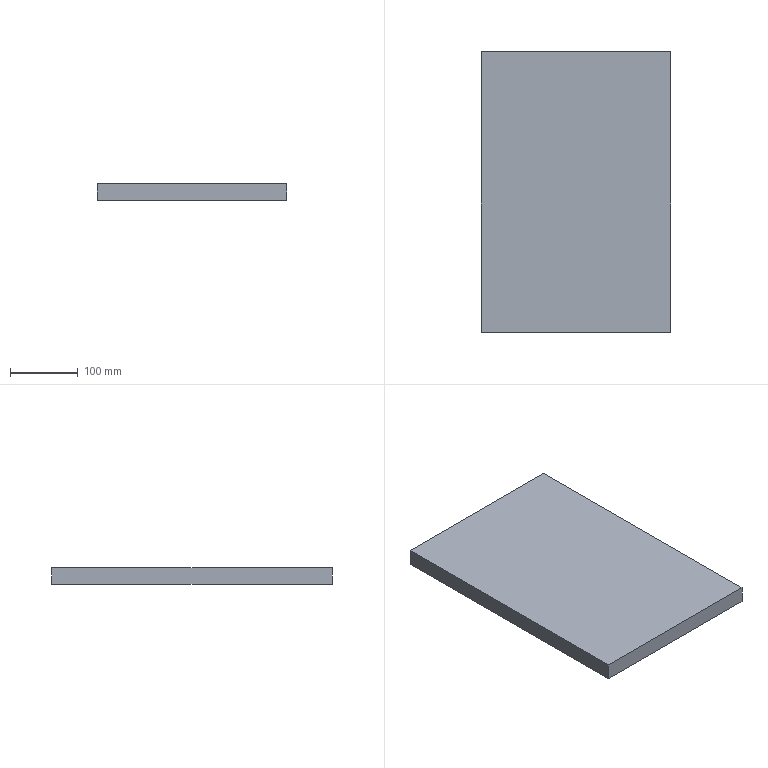Part | SolidWorks | features Extrusion 1 | 1 solid | 6 faces | box 280 x 415 x 25 mm | volume 2905000 mm3 | plane 6
STEP:
#1=CARTESIAN_POINT('',(140.,-207.5,0.));
#2=VERTEX_POINT('',#1);
#3=CARTESIAN_POINT('',(140.,207.5,0.));
#4=VERTEX_POINT('',#3);
#5=CARTESIAN_POINT('',(140.,207.5,0.));
#6=DIRECTION('',(0.,1.,0.));
#7=VECTOR('',#6,1000.);
#8=LINE('',#5,#7);
#9=EDGE_CURVE('',#2,#4,#8,.T.);
#10=ORIENTED_EDGE('',*,*,#9,.T.);
#11=CARTESIAN_POINT('',(140.,207.5,25.));
#12=VERTEX_POINT('',#11);
#13=CARTESIAN_POINT('',(140.,207.5,25.));
#14=DIRECTION('',(0.,0.,-1.));
#15=VECTOR('',#14,1000.);
#16=LINE('',#13,#15);
#17=EDGE_CURVE('',#12,#4,#16,.T.);
#18=ORIENTED_EDGE('',*,*,#17,.F.);
#19=CARTESIAN_POINT('',(140.,-207.5,25.));
#20=VERTEX_POINT('',#19);
#21=CARTESIAN_POINT('',(140.,207.5,25.));
#22=DIRECTION('',(0.,1.,0.));
#23=VECTOR('',#22,1000.);
#24=LINE('',#21,#23);
#25=EDGE_CURVE('',#20,#12,#24,.T.);
#26=ORIENTED_EDGE('',*,*,#25,.F.);
#27=CARTESIAN_POINT('',(140.,-207.5,25.));
#28=DIRECTION('',(0.,0.,-1.));
#29=VECTOR('',#28,1000.);
#30=LINE('',#27,#29);
#31=EDGE_CURVE('',#20,#2,#30,.T.);
#32=ORIENTED_EDGE('',*,*,#31,.T.);
#33=EDGE_LOOP('',(#10,#18,#26,#32));
#34=FACE_OUTER_BOUND('',#33,.T.);
#35=CARTESIAN_POINT('',(140.,207.5,25.));
#36=DIRECTION('',(-1.,0.,0.));
#37=DIRECTION('',(0.,-1.,0.));
#38=AXIS2_PLACEMENT_3D('',#35,#36,#37);
#39=PLANE('',#38);
#40=ADVANCED_FACE('',(#34),#39,.F.);
#41=CARTESIAN_POINT('',(-140.,207.5,0.));
#42=VERTEX_POINT('',#41);
#43=CARTESIAN_POINT('',(-140.,207.5,0.));
#44=DIRECTION('',(-1.,0.,0.));
#45=VECTOR('',#44,1000.);
#46=LINE('',#43,#45);
#47=EDGE_CURVE('',#4,#42,#46,.T.);
#48=ORIENTED_EDGE('',*,*,#47,.T.);
#49=CARTESIAN_POINT('',(-140.,207.5,25.));
#50=VERTEX_POINT('',#49);
#51=CARTESIAN_POINT('',(-140.,207.5,25.));
#52=DIRECTION('',(0.,0.,-1.));
#53=VECTOR('',#52,1000.);
#54=LINE('',#51,#53);
#55=EDGE_CURVE('',#50,#42,#54,.T.);
#56=ORIENTED_EDGE('',*,*,#55,.F.);
#57=CARTESIAN_POINT('',(-140.,207.5,25.));
#58=DIRECTION('',(-1.,0.,0.));
#59=VECTOR('',#58,1000.);
#60=LINE('',#57,#59);
#61=EDGE_CURVE('',#12,#50,#60,.T.);
#62=ORIENTED_EDGE('',*,*,#61,.F.);
#63=ORIENTED_EDGE('',*,*,#17,.T.);
#64=EDGE_LOOP('',(#48,#56,#62,#63));
#65=FACE_OUTER_BOUND('',#64,.T.);
#66=CARTESIAN_POINT('',(-140.,207.5,25.));
#67=DIRECTION('',(0.,-1.,0.));
#68=DIRECTION('',(0.,0.,-1.));
#69=AXIS2_PLACEMENT_3D('',#66,#67,#68);
#70=PLANE('',#69);
#71=ADVANCED_FACE('',(#65),#70,.F.);
#72=CARTESIAN_POINT('',(-140.,-207.5,0.));
#73=VERTEX_POINT('',#72);
#74=CARTESIAN_POINT('',(-140.,207.5,0.));
#75=DIRECTION('',(0.,-1.,0.));
#76=VECTOR('',#75,1000.);
#77=LINE('',#74,#76);
#78=EDGE_CURVE('',#42,#73,#77,.T.);
#79=ORIENTED_EDGE('',*,*,#78,.T.);
#80=CARTESIAN_POINT('',(-140.,-207.5,25.));
#81=VERTEX_POINT('',#80);
#82=CARTESIAN_POINT('',(-140.,-207.5,25.));
#83=DIRECTION('',(0.,0.,-1.));
#84=VECTOR('',#83,1000.);
#85=LINE('',#82,#84);
#86=EDGE_CURVE('',#81,#73,#85,.T.);
#87=ORIENTED_EDGE('',*,*,#86,.F.);
#88=CARTESIAN_POINT('',(-140.,207.5,25.));
#89=DIRECTION('',(0.,-1.,0.));
#90=VECTOR('',#89,1000.);
#91=LINE('',#88,#90);
#92=EDGE_CURVE('',#50,#81,#91,.T.);
#93=ORIENTED_EDGE('',*,*,#92,.F.);
#94=ORIENTED_EDGE('',*,*,#55,.T.);
#95=EDGE_LOOP('',(#79,#87,#93,#94));
#96=FACE_OUTER_BOUND('',#95,.T.);
#97=CARTESIAN_POINT('',(-140.,207.5,25.));
#98=DIRECTION('',(1.,0.,0.));
#99=DIRECTION('',(0.,1.,0.));
#100=AXIS2_PLACEMENT_3D('',#97,#98,#99);
#101=PLANE('',#100);
#102=ADVANCED_FACE('',(#96),#101,.F.);
#103=CARTESIAN_POINT('',(-140.,-207.5,0.));
#104=DIRECTION('',(1.,0.,0.));
#105=VECTOR('',#104,1000.);
#106=LINE('',#103,#105);
#107=EDGE_CURVE('',#73,#2,#106,.T.);
#108=ORIENTED_EDGE('',*,*,#107,.T.);
#109=ORIENTED_EDGE('',*,*,#31,.F.);
#110=CARTESIAN_POINT('',(-140.,-207.5,25.));
#111=DIRECTION('',(1.,0.,0.));
#112=VECTOR('',#111,1000.);
#113=LINE('',#110,#112);
#114=EDGE_CURVE('',#81,#20,#113,.T.);
#115=ORIENTED_EDGE('',*,*,#114,.F.);
#116=ORIENTED_EDGE('',*,*,#86,.T.);
#117=EDGE_LOOP('',(#108,#109,#115,#116));
#118=FACE_OUTER_BOUND('',#117,.T.);
#119=CARTESIAN_POINT('',(-140.,-207.5,25.));
#120=DIRECTION('',(0.,1.,0.));
#121=DIRECTION('',(0.,0.,1.));
#122=AXIS2_PLACEMENT_3D('',#119,#120,#121);
#123=PLANE('',#122);
#124=ADVANCED_FACE('',(#118),#123,.F.);
#125=ORIENTED_EDGE('',*,*,#25,.T.);
#126=ORIENTED_EDGE('',*,*,#61,.T.);
#127=ORIENTED_EDGE('',*,*,#92,.T.);
#128=ORIENTED_EDGE('',*,*,#114,.T.);
#129=EDGE_LOOP('',(#125,#126,#127,#128));
#130=FACE_OUTER_BOUND('',#129,.T.);
#131=CARTESIAN_POINT('',(0.,0.,25.));
#132=DIRECTION('',(0.,0.,1.));
#133=DIRECTION('',(1.,0.,0.));
#134=AXIS2_PLACEMENT_3D('',#131,#132,#133);
#135=PLANE('',#134);
#136=ADVANCED_FACE('',(#130),#135,.T.);
#137=ORIENTED_EDGE('',*,*,#9,.F.);
#138=ORIENTED_EDGE('',*,*,#107,.F.);
#139=ORIENTED_EDGE('',*,*,#78,.F.);
#140=ORIENTED_EDGE('',*,*,#47,.F.);
#141=EDGE_LOOP('',(#137,#138,#139,#140));
#142=FACE_OUTER_BOUND('',#141,.T.);
#143=CARTESIAN_POINT('',(0.,0.,0.));
#144=DIRECTION('',(0.,0.,1.));
#145=DIRECTION('',(1.,0.,0.));
#146=AXIS2_PLACEMENT_3D('',#143,#144,#145);
#147=PLANE('',#146);
#148=ADVANCED_FACE('',(#142),#147,.F.);
#149=CLOSED_SHELL('',(#40,#71,#102,#124,#136,#148));
#150=MANIFOLD_SOLID_BREP('',#149);
#151=CARTESIAN_POINT('',(0.,0.,0.));
#152=DIRECTION('',(0.,0.,1.));
#153=DIRECTION('',(1.,0.,0.));
#154=AXIS2_PLACEMENT_3D('',#151,#152,#153);
#155=(LENGTH_UNIT()NAMED_UNIT(*)SI_UNIT(.MILLI.,.METRE.));
#156=UNCERTAINTY_MEASURE_WITH_UNIT(LENGTH_MEASURE(0.00001),#155,'','');
#157=(NAMED_UNIT(*)PLANE_ANGLE_UNIT()SI_UNIT($,.RADIAN.));
#158=(NAMED_UNIT(*)SI_UNIT($,.STERADIAN.)SOLID_ANGLE_UNIT());
#159=(GEOMETRIC_REPRESENTATION_CONTEXT(3)GLOBAL_UNCERTAINTY_ASSIGNED_CONTEXT((#156))GLOBAL_UNIT_ASSIGNED_CONTEXT((#155,#157,#158))REPRESENTATION_CONTEXT('',''));
#160=ADVANCED_BREP_SHAPE_REPRESENTATION('',(#150,#154),#159);